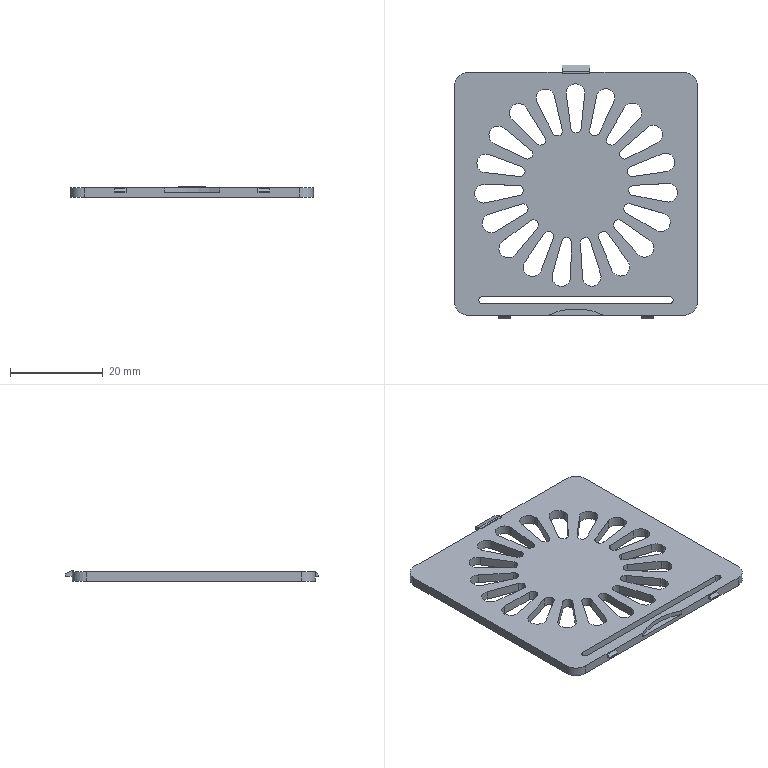Part | SolidWorks | features ICE 4, Extrusion 1, MirrorPattern 1 | 1 solid | 132 faces | box 52.5 x 54.75 x 2.2 mm | volume 4171 mm3 | cylinder 66 | plane 66 | commonest cylinder face diameters 4 x30 2.2 x28 6 x4 1.5 x3 27 x1